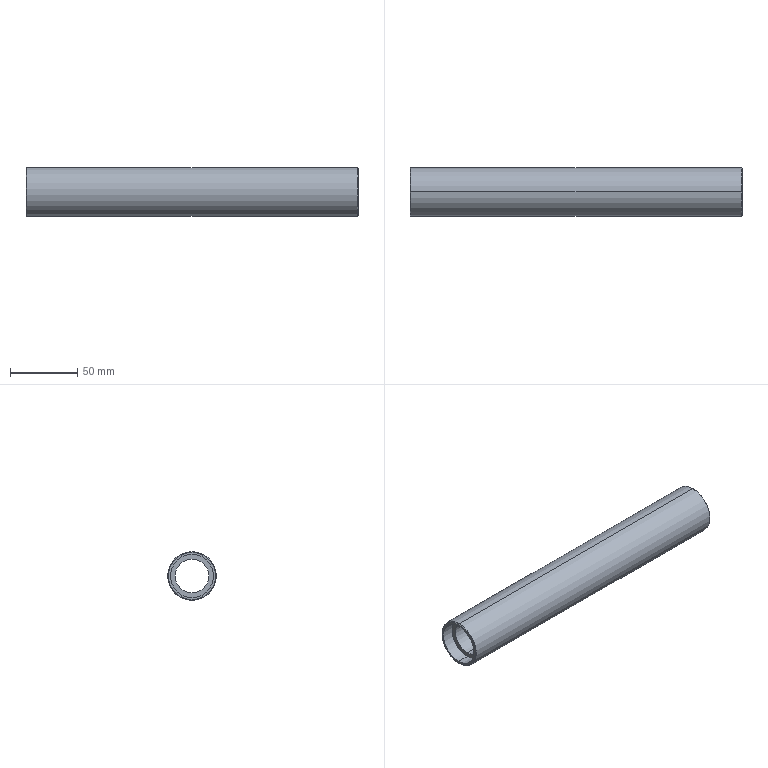Part | STEP file | 1 solid | 16 faces | box 246 x 36 x 36 mm | volume 123974 mm3 | cylinder 8 | cone 4 | plane 4 | commonest cylinder face diameters 32 x4 25 x2 36 x2
STEP:
#1=CARTESIAN_POINT('',(0.,0.,0.));
#2=DIRECTION('',(0.,0.,1.));
#3=DIRECTION('',(1.,0.,0.));
#4=AXIS2_PLACEMENT_3D('',#1,#2,#3);
#5=CARTESIAN_POINT('',(-123.,0.,17.5));
#6=VERTEX_POINT('',#5);
#7=CARTESIAN_POINT('',(-123.,0.,-17.5));
#8=VERTEX_POINT('',#7);
#9=CARTESIAN_POINT('',(-123.,0.,0.));
#10=DIRECTION('',(-1.,0.,0.));
#11=DIRECTION('',(0.,0.,-1.));
#12=AXIS2_PLACEMENT_3D('',#9,#10,#11);
#13=CIRCLE('',#12,17.5);
#14=CARTESIAN_POINT('',(-123.,0.,0.));
#15=DIRECTION('',(1.,0.,0.));
#16=DIRECTION('',(0.,0.,-1.));
#17=AXIS2_PLACEMENT_3D('',#14,#15,#16);
#18=CONICAL_SURFACE('',#17,17.5,0.7854);
#19=CARTESIAN_POINT('',(6.283,0.));
#20=DIRECTION('',(-1.,0.));
#21=VECTOR('',#20,1.);
#22=LINE('',#19,#21);
#23=(GEOMETRIC_REPRESENTATION_CONTEXT(2)PARAMETRIC_REPRESENTATION_CONTEXT()REPRESENTATION_CONTEXT('',''));
#24=DEFINITIONAL_REPRESENTATION('',(#22),#23);
#25=PCURVE('',#18,#24);
#26=CARTESIAN_POINT('',(-123.,18.,0.));
#27=DIRECTION('',(1.,0.,0.));
#28=DIRECTION('',(0.,0.,-1.));
#29=AXIS2_PLACEMENT_3D('',#26,#27,#28);
#30=PLANE('',#29);
#31=CARTESIAN_POINT('',(17.5,-18.));
#32=CARTESIAN_POINT('',(17.5,-48.311));
#33=CARTESIAN_POINT('',(-8.75,-33.155));
#34=CARTESIAN_POINT('',(-35.,-18.));
#35=CARTESIAN_POINT('',(-8.75,-2.845));
#36=CARTESIAN_POINT('',(17.5,12.311));
#37=CARTESIAN_POINT('',(17.5,-18.));
#38=(BOUNDED_CURVE()B_SPLINE_CURVE(2,(#31,#32,#33,#34,#35,#36,#37),.UNSPECIFIED.,.T.,.F.)B_SPLINE_CURVE_WITH_KNOTS((1,2,2,2,2,1),(-2.094,0.,2.094,4.189,6.283,8.378),.UNSPECIFIED.)CURVE()GEOMETRIC_REPRESENTATION_ITEM()RATIONAL_B_SPLINE_CURVE((1.,0.5,1.,0.5,1.,0.5,1.))REPRESENTATION_ITEM(''));
#39=(GEOMETRIC_REPRESENTATION_CONTEXT(2)PARAMETRIC_REPRESENTATION_CONTEXT()REPRESENTATION_CONTEXT('',''));
#40=DEFINITIONAL_REPRESENTATION('',(#38),#39);
#41=PCURVE('',#30,#40);
#42=SURFACE_CURVE('',#13,(#25,#41),.PCURVE_S1.);
#43=EDGE_CURVE('',#6,#8,#42,.T.);
#44=ORIENTED_EDGE('',*,*,#43,.F.);
#45=CARTESIAN_POINT('',(-122.5,0.,18.));
#46=VERTEX_POINT('',#45);
#47=CARTESIAN_POINT('',(-123.,0.,17.5));
#48=DIRECTION('',(0.7071,0.,0.7071));
#49=VECTOR('',#48,1.);
#50=LINE('',#47,#49);
#51=CARTESIAN_POINT('',(3.142,0.));
#52=DIRECTION('',(0.,1.));
#53=VECTOR('',#52,1.);
#54=LINE('',#51,#53);
#55=(GEOMETRIC_REPRESENTATION_CONTEXT(2)PARAMETRIC_REPRESENTATION_CONTEXT()REPRESENTATION_CONTEXT('',''));
#56=DEFINITIONAL_REPRESENTATION('',(#54),#55);
#57=PCURVE('',#18,#56);
#58=CARTESIAN_POINT('',(-123.,0.,0.));
#59=DIRECTION('',(1.,0.,0.));
#60=DIRECTION('',(0.,0.,-1.));
#61=AXIS2_PLACEMENT_3D('',#58,#59,#60);
#62=CONICAL_SURFACE('',#61,17.5,0.7854);
#63=CARTESIAN_POINT('',(3.142,0.));
#64=DIRECTION('',(0.,1.));
#65=VECTOR('',#64,1.);
#66=LINE('',#63,#65);
#67=(GEOMETRIC_REPRESENTATION_CONTEXT(2)PARAMETRIC_REPRESENTATION_CONTEXT()REPRESENTATION_CONTEXT('',''));
#68=DEFINITIONAL_REPRESENTATION('',(#66),#67);
#69=PCURVE('',#62,#68);
#70=SURFACE_CURVE('',#50,(#57,#69),.PCURVE_S1.);
#71=EDGE_CURVE('',#6,#46,#70,.T.);
#72=ORIENTED_EDGE('',*,*,#71,.T.);
#73=CARTESIAN_POINT('',(-122.5,0.,-18.));
#74=VERTEX_POINT('',#73);
#75=CARTESIAN_POINT('',(-122.5,0.,0.));
#76=DIRECTION('',(1.,0.,0.));
#77=DIRECTION('',(0.,0.,-1.));
#78=AXIS2_PLACEMENT_3D('',#75,#76,#77);
#79=CIRCLE('',#78,18.);
#80=CARTESIAN_POINT('',(0.,0.5));
#81=DIRECTION('',(1.,0.));
#82=VECTOR('',#81,1.);
#83=LINE('',#80,#82);
#84=(GEOMETRIC_REPRESENTATION_CONTEXT(2)PARAMETRIC_REPRESENTATION_CONTEXT()REPRESENTATION_CONTEXT('',''));
#85=DEFINITIONAL_REPRESENTATION('',(#83),#84);
#86=PCURVE('',#18,#85);
#87=CARTESIAN_POINT('',(0.,0.,0.));
#88=DIRECTION('',(-1.,0.,0.));
#89=DIRECTION('',(0.,0.,1.));
#90=AXIS2_PLACEMENT_3D('',#87,#88,#89);
#91=CYLINDRICAL_SURFACE('',#90,18.);
#92=CARTESIAN_POINT('',(3.142,122.5));
#93=DIRECTION('',(-1.,0.));
#94=VECTOR('',#93,1.);
#95=LINE('',#92,#94);
#96=(GEOMETRIC_REPRESENTATION_CONTEXT(2)PARAMETRIC_REPRESENTATION_CONTEXT()REPRESENTATION_CONTEXT('',''));
#97=DEFINITIONAL_REPRESENTATION('',(#95),#96);
#98=PCURVE('',#91,#97);
#99=SURFACE_CURVE('',#79,(#86,#98),.PCURVE_S1.);
#100=EDGE_CURVE('',#74,#46,#99,.T.);
#101=ORIENTED_EDGE('',*,*,#100,.F.);
#102=CARTESIAN_POINT('',(-123.,0.,-17.5));
#103=DIRECTION('',(0.7071,0.,-0.7071));
#104=VECTOR('',#103,1.);
#105=LINE('',#102,#104);
#106=CARTESIAN_POINT('',(0.,0.));
#107=DIRECTION('',(0.,1.));
#108=VECTOR('',#107,1.);
#109=LINE('',#106,#108);
#110=(GEOMETRIC_REPRESENTATION_CONTEXT(2)PARAMETRIC_REPRESENTATION_CONTEXT()REPRESENTATION_CONTEXT('',''));
#111=DEFINITIONAL_REPRESENTATION('',(#109),#110);
#112=PCURVE('',#18,#111);
#113=CARTESIAN_POINT('',(6.283,0.));
#114=DIRECTION('',(0.,1.));
#115=VECTOR('',#114,1.);
#116=LINE('',#113,#115);
#117=(GEOMETRIC_REPRESENTATION_CONTEXT(2)PARAMETRIC_REPRESENTATION_CONTEXT()REPRESENTATION_CONTEXT('',''));
#118=DEFINITIONAL_REPRESENTATION('',(#116),#117);
#119=PCURVE('',#62,#118);
#120=SURFACE_CURVE('',#105,(#112,#119),.PCURVE_S1.);
#121=EDGE_CURVE('',#8,#74,#120,.T.);
#122=ORIENTED_EDGE('',*,*,#121,.F.);
#123=EDGE_LOOP('',(#44,#72,#101,#122));
#124=FACE_BOUND('',#123,.T.);
#125=ADVANCED_FACE('',(#124),#18,.T.);
#126=CARTESIAN_POINT('',(123.,0.,-17.5));
#127=VERTEX_POINT('',#126);
#128=CARTESIAN_POINT('',(123.,0.,17.5));
#129=VERTEX_POINT('',#128);
#130=CARTESIAN_POINT('',(123.,0.,0.));
#131=DIRECTION('',(1.,0.,0.));
#132=DIRECTION('',(0.,0.,1.));
#133=AXIS2_PLACEMENT_3D('',#130,#131,#132);
#134=CIRCLE('',#133,17.5);
#135=CARTESIAN_POINT('',(122.5,0.,0.));
#136=DIRECTION('',(-1.,0.,0.));
#137=DIRECTION('',(0.,0.,1.));
#138=AXIS2_PLACEMENT_3D('',#135,#136,#137);
#139=CONICAL_SURFACE('',#138,18.,0.7854);
#140=CARTESIAN_POINT('',(6.283,-0.5));
#141=DIRECTION('',(-1.,0.));
#142=VECTOR('',#141,1.);
#143=LINE('',#140,#142);
#144=(GEOMETRIC_REPRESENTATION_CONTEXT(2)PARAMETRIC_REPRESENTATION_CONTEXT()REPRESENTATION_CONTEXT('',''));
#145=DEFINITIONAL_REPRESENTATION('',(#143),#144);
#146=PCURVE('',#139,#145);
#147=CARTESIAN_POINT('',(123.,18.,0.));
#148=DIRECTION('',(-1.,0.,0.));
#149=DIRECTION('',(0.,0.,1.));
#150=AXIS2_PLACEMENT_3D('',#147,#148,#149);
#151=PLANE('',#150);
#152=CARTESIAN_POINT('',(17.5,-18.));
#153=CARTESIAN_POINT('',(17.5,-48.311));
#154=CARTESIAN_POINT('',(-8.75,-33.155));
#155=CARTESIAN_POINT('',(-35.,-18.));
#156=CARTESIAN_POINT('',(-8.75,-2.845));
#157=CARTESIAN_POINT('',(17.5,12.311));
#158=CARTESIAN_POINT('',(17.5,-18.));
#159=(BOUNDED_CURVE()B_SPLINE_CURVE(2,(#152,#153,#154,#155,#156,#157,#158),.UNSPECIFIED.,.T.,.F.)B_SPLINE_CURVE_WITH_KNOTS((1,2,2,2,2,1),(-2.094,0.,2.094,4.189,6.283,8.378),.UNSPECIFIED.)CURVE()GEOMETRIC_REPRESENTATION_ITEM()RATIONAL_B_SPLINE_CURVE((1.,0.5,1.,0.5,1.,0.5,1.))REPRESENTATION_ITEM(''));
#160=(GEOMETRIC_REPRESENTATION_CONTEXT(2)PARAMETRIC_REPRESENTATION_CONTEXT()REPRESENTATION_CONTEXT('',''));
#161=DEFINITIONAL_REPRESENTATION('',(#159),#160);
#162=PCURVE('',#151,#161);
#163=SURFACE_CURVE('',#134,(#146,#162),.PCURVE_S1.);
#164=EDGE_CURVE('',#127,#129,#163,.T.);
#165=ORIENTED_EDGE('',*,*,#164,.F.);
#166=CARTESIAN_POINT('',(122.5,0.,-18.));
#167=VERTEX_POINT('',#166);
#168=CARTESIAN_POINT('',(122.5,0.,-18.));
#169=DIRECTION('',(-0.7071,0.,-0.7071));
#170=VECTOR('',#169,1.);
#171=LINE('',#168,#170);
#172=CARTESIAN_POINT('',(3.142,0.));
#173=DIRECTION('',(0.,1.));
#174=VECTOR('',#173,1.);
#175=LINE('',#172,#174);
#176=(GEOMETRIC_REPRESENTATION_CONTEXT(2)PARAMETRIC_REPRESENTATION_CONTEXT()REPRESENTATION_CONTEXT('',''));
#177=DEFINITIONAL_REPRESENTATION('',(#175),#176);
#178=PCURVE('',#139,#177);
#179=CARTESIAN_POINT('',(122.5,0.,0.));
#180=DIRECTION('',(-1.,0.,0.));
#181=DIRECTION('',(0.,0.,1.));
#182=AXIS2_PLACEMENT_3D('',#179,#180,#181);
#183=CONICAL_SURFACE('',#182,18.,0.7854);
#184=CARTESIAN_POINT('',(3.142,0.));
#185=DIRECTION('',(0.,1.));
#186=VECTOR('',#185,1.);
#187=LINE('',#184,#186);
#188=(GEOMETRIC_REPRESENTATION_CONTEXT(2)PARAMETRIC_REPRESENTATION_CONTEXT()REPRESENTATION_CONTEXT('',''));
#189=DEFINITIONAL_REPRESENTATION('',(#187),#188);
#190=PCURVE('',#183,#189);
#191=SURFACE_CURVE('',#171,(#178,#190),.PCURVE_S1.);
#192=EDGE_CURVE('',#127,#167,#191,.T.);
#193=ORIENTED_EDGE('',*,*,#192,.T.);
#194=CARTESIAN_POINT('',(122.5,0.,18.));
#195=VERTEX_POINT('',#194);
#196=CARTESIAN_POINT('',(122.5,0.,0.));
#197=DIRECTION('',(-1.,0.,0.));
#198=DIRECTION('',(0.,0.,1.));
#199=AXIS2_PLACEMENT_3D('',#196,#197,#198);
#200=CIRCLE('',#199,18.);
#201=CARTESIAN_POINT('',(0.,0.));
#202=DIRECTION('',(1.,0.));
#203=VECTOR('',#202,1.);
#204=LINE('',#201,#203);
#205=(GEOMETRIC_REPRESENTATION_CONTEXT(2)PARAMETRIC_REPRESENTATION_CONTEXT()REPRESENTATION_CONTEXT('',''));
#206=DEFINITIONAL_REPRESENTATION('',(#204),#205);
#207=PCURVE('',#139,#206);
#208=CARTESIAN_POINT('',(0.,-122.5));
#209=DIRECTION('',(1.,0.));
#210=VECTOR('',#209,1.);
#211=LINE('',#208,#210);
#212=(GEOMETRIC_REPRESENTATION_CONTEXT(2)PARAMETRIC_REPRESENTATION_CONTEXT()REPRESENTATION_CONTEXT('',''));
#213=DEFINITIONAL_REPRESENTATION('',(#211),#212);
#214=PCURVE('',#91,#213);
#215=SURFACE_CURVE('',#200,(#207,#214),.PCURVE_S1.);
#216=EDGE_CURVE('',#195,#167,#215,.T.);
#217=ORIENTED_EDGE('',*,*,#216,.F.);
#218=CARTESIAN_POINT('',(122.5,0.,18.));
#219=DIRECTION('',(-0.7071,0.,0.7071));
#220=VECTOR('',#219,1.);
#221=LINE('',#218,#220);
#222=CARTESIAN_POINT('',(0.,0.));
#223=DIRECTION('',(0.,1.));
#224=VECTOR('',#223,1.);
#225=LINE('',#222,#224);
#226=(GEOMETRIC_REPRESENTATION_CONTEXT(2)PARAMETRIC_REPRESENTATION_CONTEXT()REPRESENTATION_CONTEXT('',''));
#227=DEFINITIONAL_REPRESENTATION('',(#225),#226);
#228=PCURVE('',#139,#227);
#229=CARTESIAN_POINT('',(6.283,0.));
#230=DIRECTION('',(0.,1.));
#231=VECTOR('',#230,1.);
#232=LINE('',#229,#231);
#233=(GEOMETRIC_REPRESENTATION_CONTEXT(2)PARAMETRIC_REPRESENTATION_CONTEXT()REPRESENTATION_CONTEXT('',''));
#234=DEFINITIONAL_REPRESENTATION('',(#232),#233);
#235=PCURVE('',#183,#234);
#236=SURFACE_CURVE('',#221,(#228,#235),.PCURVE_S1.);
#237=EDGE_CURVE('',#129,#195,#236,.T.);
#238=ORIENTED_EDGE('',*,*,#237,.F.);
#239=EDGE_LOOP('',(#165,#193,#217,#238));
#240=FACE_BOUND('',#239,.T.);
#241=ADVANCED_FACE('',(#240),#139,.T.);
#242=CARTESIAN_POINT('',(114.,0.,12.5));
#243=VERTEX_POINT('',#242);
#244=CARTESIAN_POINT('',(-114.,0.,12.5));
#245=VERTEX_POINT('',#244);
#246=CARTESIAN_POINT('',(0.,0.,12.5));
#247=DIRECTION('',(-1.,0.,0.));
#248=VECTOR('',#247,1.);
#249=LINE('',#246,#248);
#250=CARTESIAN_POINT('',(0.,0.,0.));
#251=DIRECTION('',(-1.,0.,0.));
#252=DIRECTION('',(0.,0.,1.));
#253=AXIS2_PLACEMENT_3D('',#250,#251,#252);
#254=CYLINDRICAL_SURFACE('',#253,12.5);
#255=CARTESIAN_POINT('',(6.283,0.));
#256=DIRECTION('',(0.,1.));
#257=VECTOR('',#256,1.);
#258=LINE('',#255,#257);
#259=(GEOMETRIC_REPRESENTATION_CONTEXT(2)PARAMETRIC_REPRESENTATION_CONTEXT()REPRESENTATION_CONTEXT('',''));
#260=DEFINITIONAL_REPRESENTATION('',(#258),#259);
#261=PCURVE('',#254,#260);
#262=CARTESIAN_POINT('',(0.,0.,0.));
#263=DIRECTION('',(-1.,0.,0.));
#264=DIRECTION('',(0.,0.,1.));
#265=AXIS2_PLACEMENT_3D('',#262,#263,#264);
#266=CYLINDRICAL_SURFACE('',#265,12.5);
#267=CARTESIAN_POINT('',(0.,0.));
#268=DIRECTION('',(0.,1.));
#269=VECTOR('',#268,1.);
#270=LINE('',#267,#269);
#271=(GEOMETRIC_REPRESENTATION_CONTEXT(2)PARAMETRIC_REPRESENTATION_CONTEXT()REPRESENTATION_CONTEXT('',''));
#272=DEFINITIONAL_REPRESENTATION('',(#270),#271);
#273=PCURVE('',#266,#272);
#274=SURFACE_CURVE('',#249,(#261,#273),.PCURVE_S1.);
#275=EDGE_CURVE('',#243,#245,#274,.T.);
#276=ORIENTED_EDGE('',*,*,#275,.T.);
#277=CARTESIAN_POINT('',(-114.,0.,-12.5));
#278=VERTEX_POINT('',#277);
#279=CARTESIAN_POINT('',(-114.,0.,0.));
#280=DIRECTION('',(-1.,0.,0.));
#281=DIRECTION('',(0.,0.,1.));
#282=AXIS2_PLACEMENT_3D('',#279,#280,#281);
#283=CIRCLE('',#282,12.5);
#284=CARTESIAN_POINT('',(0.,114.));
#285=DIRECTION('',(1.,0.));
#286=VECTOR('',#285,1.);
#287=LINE('',#284,#286);
#288=(GEOMETRIC_REPRESENTATION_CONTEXT(2)PARAMETRIC_REPRESENTATION_CONTEXT()REPRESENTATION_CONTEXT('',''));
#289=DEFINITIONAL_REPRESENTATION('',(#287),#288);
#290=PCURVE('',#254,#289);
#291=CARTESIAN_POINT('',(-114.,16.,0.));
#292=DIRECTION('',(1.,0.,0.));
#293=DIRECTION('',(0.,0.,-1.));
#294=AXIS2_PLACEMENT_3D('',#291,#292,#293);
#295=PLANE('',#294);
#296=CARTESIAN_POINT('',(-12.5,-16.));
#297=CARTESIAN_POINT('',(-12.5,5.651));
#298=CARTESIAN_POINT('',(6.25,-5.175));
#299=CARTESIAN_POINT('',(25.,-16.));
#300=CARTESIAN_POINT('',(6.25,-26.825));
#301=CARTESIAN_POINT('',(-12.5,-37.651));
#302=CARTESIAN_POINT('',(-12.5,-16.));
#303=(BOUNDED_CURVE()B_SPLINE_CURVE(2,(#296,#297,#298,#299,#300,#301,#302),.UNSPECIFIED.,.T.,.F.)B_SPLINE_CURVE_WITH_KNOTS((1,2,2,2,2,1),(-2.094,0.,2.094,4.189,6.283,8.378),.UNSPECIFIED.)CURVE()GEOMETRIC_REPRESENTATION_ITEM()RATIONAL_B_SPLINE_CURVE((1.,0.5,1.,0.5,1.,0.5,1.))REPRESENTATION_ITEM(''));
#304=(GEOMETRIC_REPRESENTATION_CONTEXT(2)PARAMETRIC_REPRESENTATION_CONTEXT()REPRESENTATION_CONTEXT('',''));
#305=DEFINITIONAL_REPRESENTATION('',(#303),#304);
#306=PCURVE('',#295,#305);
#307=SURFACE_CURVE('',#283,(#290,#306),.PCURVE_S1.);
#308=EDGE_CURVE('',#278,#245,#307,.T.);
#309=ORIENTED_EDGE('',*,*,#308,.F.);
#310=CARTESIAN_POINT('',(114.,0.,-12.5));
#311=VERTEX_POINT('',#310);
#312=CARTESIAN_POINT('',(0.,0.,-12.5));
#313=DIRECTION('',(-1.,0.,0.));
#314=VECTOR('',#313,1.);
#315=LINE('',#312,#314);
#316=CARTESIAN_POINT('',(3.142,0.));
#317=DIRECTION('',(0.,1.));
#318=VECTOR('',#317,1.);
#319=LINE('',#316,#318);
#320=(GEOMETRIC_REPRESENTATION_CONTEXT(2)PARAMETRIC_REPRESENTATION_CONTEXT()REPRESENTATION_CONTEXT('',''));
#321=DEFINITIONAL_REPRESENTATION('',(#319),#320);
#322=PCURVE('',#254,#321);
#323=CARTESIAN_POINT('',(3.142,0.));
#324=DIRECTION('',(0.,1.));
#325=VECTOR('',#324,1.);
#326=LINE('',#323,#325);
#327=(GEOMETRIC_REPRESENTATION_CONTEXT(2)PARAMETRIC_REPRESENTATION_CONTEXT()REPRESENTATION_CONTEXT('',''));
#328=DEFINITIONAL_REPRESENTATION('',(#326),#327);
#329=PCURVE('',#266,#328);
#330=SURFACE_CURVE('',#315,(#322,#329),.PCURVE_S1.);
#331=EDGE_CURVE('',#311,#278,#330,.T.);
#332=ORIENTED_EDGE('',*,*,#331,.F.);
#333=CARTESIAN_POINT('',(114.,0.,0.));
#334=DIRECTION('',(-1.,0.,0.));
#335=DIRECTION('',(0.,0.,1.));
#336=AXIS2_PLACEMENT_3D('',#333,#334,#335);
#337=CIRCLE('',#336,12.5);
#338=CARTESIAN_POINT('',(0.,-114.));
#339=DIRECTION('',(1.,0.));
#340=VECTOR('',#339,1.);
#341=LINE('',#338,#340);
#342=(GEOMETRIC_REPRESENTATION_CONTEXT(2)PARAMETRIC_REPRESENTATION_CONTEXT()REPRESENTATION_CONTEXT('',''));
#343=DEFINITIONAL_REPRESENTATION('',(#341),#342);
#344=PCURVE('',#254,#343);
#345=CARTESIAN_POINT('',(114.,16.,0.));
#346=DIRECTION('',(-1.,0.,0.));
#347=DIRECTION('',(0.,0.,1.));
#348=AXIS2_PLACEMENT_3D('',#345,#346,#347);
#349=PLANE('',#348);
#350=CARTESIAN_POINT('',(0.,-16.));
#351=DIRECTION('',(1.,0.));
#352=AXIS2_PLACEMENT_2D('',#350,#351);
#353=CIRCLE('',#352,12.5);
#354=(GEOMETRIC_REPRESENTATION_CONTEXT(2)PARAMETRIC_REPRESENTATION_CONTEXT()REPRESENTATION_CONTEXT('',''));
#355=DEFINITIONAL_REPRESENTATION('',(#353),#354);
#356=PCURVE('',#349,#355);
#357=SURFACE_CURVE('',#337,(#344,#356),.PCURVE_S1.);
#358=EDGE_CURVE('',#311,#243,#357,.T.);
#359=ORIENTED_EDGE('',*,*,#358,.T.);
#360=EDGE_LOOP('',(#276,#309,#332,#359));
#361=FACE_BOUND('',#360,.F.);
#362=ADVANCED_FACE('',(#361),#254,.F.);
#363=CARTESIAN_POINT('',(123.,0.,16.));
#364=VERTEX_POINT('',#363);
#365=CARTESIAN_POINT('',(114.,0.,16.));
#366=VERTEX_POINT('',#365);
#367=CARTESIAN_POINT('',(0.,0.,16.));
#368=DIRECTION('',(-1.,0.,0.));
#369=VECTOR('',#368,1.);
#370=LINE('',#367,#369);
#371=CARTESIAN_POINT('',(0.,0.,0.));
#372=DIRECTION('',(-1.,0.,0.));
#373=DIRECTION('',(0.,0.,1.));
#374=AXIS2_PLACEMENT_3D('',#371,#372,#373);
#375=CYLINDRICAL_SURFACE('',#374,16.);
#376=CARTESIAN_POINT('',(6.283,0.));
#377=DIRECTION('',(0.,1.));
#378=VECTOR('',#377,1.);
#379=LINE('',#376,#378);
#380=(GEOMETRIC_REPRESENTATION_CONTEXT(2)PARAMETRIC_REPRESENTATION_CONTEXT()REPRESENTATION_CONTEXT('',''));
#381=DEFINITIONAL_REPRESENTATION('',(#379),#380);
#382=PCURVE('',#375,#381);
#383=CARTESIAN_POINT('',(0.,0.,0.));
#384=DIRECTION('',(-1.,0.,0.));
#385=DIRECTION('',(0.,0.,1.));
#386=AXIS2_PLACEMENT_3D('',#383,#384,#385);
#387=CYLINDRICAL_SURFACE('',#386,16.);
#388=CARTESIAN_POINT('',(0.,0.));
#389=DIRECTION('',(0.,1.));
#390=VECTOR('',#389,1.);
#391=LINE('',#388,#390);
#392=(GEOMETRIC_REPRESENTATION_CONTEXT(2)PARAMETRIC_REPRESENTATION_CONTEXT()REPRESENTATION_CONTEXT('',''));
#393=DEFINITIONAL_REPRESENTATION('',(#391),#392);
#394=PCURVE('',#387,#393);
#395=SURFACE_CURVE('',#370,(#382,#394),.PCURVE_S1.);
#396=EDGE_CURVE('',#364,#366,#395,.T.);
#397=ORIENTED_EDGE('',*,*,#396,.T.);
#398=CARTESIAN_POINT('',(114.,0.,-16.));
#399=VERTEX_POINT('',#398);
#400=CARTESIAN_POINT('',(114.,0.,0.));
#401=DIRECTION('',(-1.,0.,0.));
#402=DIRECTION('',(0.,0.,1.));
#403=AXIS2_PLACEMENT_3D('',#400,#401,#402);
#404=CIRCLE('',#403,16.);
#405=CARTESIAN_POINT('',(0.,-114.));
#406=DIRECTION('',(1.,0.));
#407=VECTOR('',#406,1.);
#408=LINE('',#405,#407);
#409=(GEOMETRIC_REPRESENTATION_CONTEXT(2)PARAMETRIC_REPRESENTATION_CONTEXT()REPRESENTATION_CONTEXT('',''));
#410=DEFINITIONAL_REPRESENTATION('',(#408),#409);
#411=PCURVE('',#375,#410);
#412=CARTESIAN_POINT('',(0.,-16.));
#413=DIRECTION('',(1.,0.));
#414=AXIS2_PLACEMENT_2D('',#412,#413);
#415=CIRCLE('',#414,16.);
#416=(GEOMETRIC_REPRESENTATION_CONTEXT(2)PARAMETRIC_REPRESENTATION_CONTEXT()REPRESENTATION_CONTEXT('',''));
#417=DEFINITIONAL_REPRESENTATION('',(#415),#416);
#418=PCURVE('',#349,#417);
#419=SURFACE_CURVE('',#404,(#411,#418),.PCURVE_S1.);
#420=EDGE_CURVE('',#399,#366,#419,.T.);
#421=ORIENTED_EDGE('',*,*,#420,.F.);
#422=CARTESIAN_POINT('',(123.,0.,-16.));
#423=VERTEX_POINT('',#422);
#424=CARTESIAN_POINT('',(0.,0.,-16.));
#425=DIRECTION('',(-1.,0.,0.));
#426=VECTOR('',#425,1.);
#427=LINE('',#424,#426);
#428=CARTESIAN_POINT('',(3.142,0.));
#429=DIRECTION('',(0.,1.));
#430=VECTOR('',#429,1.);
#431=LINE('',#428,#430);
#432=(GEOMETRIC_REPRESENTATION_CONTEXT(2)PARAMETRIC_REPRESENTATION_CONTEXT()REPRESENTATION_CONTEXT('',''));
#433=DEFINITIONAL_REPRESENTATION('',(#431),#432);
#434=PCURVE('',#375,#433);
#435=CARTESIAN_POINT('',(3.142,0.));
#436=DIRECTION('',(0.,1.));
#437=VECTOR('',#436,1.);
#438=LINE('',#435,#437);
#439=(GEOMETRIC_REPRESENTATION_CONTEXT(2)PARAMETRIC_REPRESENTATION_CONTEXT()REPRESENTATION_CONTEXT('',''));
#440=DEFINITIONAL_REPRESENTATION('',(#438),#439);
#441=PCURVE('',#387,#440);
#442=SURFACE_CURVE('',#427,(#434,#441),.PCURVE_S1.);
#443=EDGE_CURVE('',#423,#399,#442,.T.);
#444=ORIENTED_EDGE('',*,*,#443,.F.);
#445=CARTESIAN_POINT('',(123.,0.,0.));
#446=DIRECTION('',(-1.,0.,0.));
#447=DIRECTION('',(0.,0.,1.));
#448=AXIS2_PLACEMENT_3D('',#445,#446,#447);
#449=CIRCLE('',#448,16.);
#450=CARTESIAN_POINT('',(0.,-123.));
#451=DIRECTION('',(1.,0.));
#452=VECTOR('',#451,1.);
#453=LINE('',#450,#452);
#454=(GEOMETRIC_REPRESENTATION_CONTEXT(2)PARAMETRIC_REPRESENTATION_CONTEXT()REPRESENTATION_CONTEXT('',''));
#455=DEFINITIONAL_REPRESENTATION('',(#453),#454);
#456=PCURVE('',#375,#455);
#457=CARTESIAN_POINT('',(0.,-18.));
#458=DIRECTION('',(1.,0.));
#459=AXIS2_PLACEMENT_2D('',#457,#458);
#460=CIRCLE('',#459,16.);
#461=(GEOMETRIC_REPRESENTATION_CONTEXT(2)PARAMETRIC_REPRESENTATION_CONTEXT()REPRESENTATION_CONTEXT('',''));
#462=DEFINITIONAL_REPRESENTATION('',(#460),#461);
#463=PCURVE('',#151,#462);
#464=SURFACE_CURVE('',#449,(#456,#463),.PCURVE_S1.);
#465=EDGE_CURVE('',#423,#364,#464,.T.);
#466=ORIENTED_EDGE('',*,*,#465,.T.);
#467=EDGE_LOOP('',(#397,#421,#444,#466));
#468=FACE_BOUND('',#467,.F.);
#469=ADVANCED_FACE('',(#468),#375,.F.);
#470=ORIENTED_EDGE('',*,*,#216,.T.);
#471=CARTESIAN_POINT('',(0.,0.,-18.));
#472=DIRECTION('',(-1.,0.,0.));
#473=VECTOR('',#472,1.);
#474=LINE('',#471,#473);
#475=CARTESIAN_POINT('',(3.142,0.));
#476=DIRECTION('',(0.,1.));
#477=VECTOR('',#476,1.);
#478=LINE('',#475,#477);
#479=(GEOMETRIC_REPRESENTATION_CONTEXT(2)PARAMETRIC_REPRESENTATION_CONTEXT()REPRESENTATION_CONTEXT('',''));
#480=DEFINITIONAL_REPRESENTATION('',(#478),#479);
#481=PCURVE('',#91,#480);
#482=CARTESIAN_POINT('',(0.,0.,0.));
#483=DIRECTION('',(-1.,0.,0.));
#484=DIRECTION('',(0.,0.,1.));
#485=AXIS2_PLACEMENT_3D('',#482,#483,#484);
#486=CYLINDRICAL_SURFACE('',#485,18.);
#487=CARTESIAN_POINT('',(3.142,0.));
#488=DIRECTION('',(0.,1.));
#489=VECTOR('',#488,1.);
#490=LINE('',#487,#489);
#491=(GEOMETRIC_REPRESENTATION_CONTEXT(2)PARAMETRIC_REPRESENTATION_CONTEXT()REPRESENTATION_CONTEXT('',''));
#492=DEFINITIONAL_REPRESENTATION('',(#490),#491);
#493=PCURVE('',#486,#492);
#494=SURFACE_CURVE('',#474,(#481,#493),.PCURVE_S1.);
#495=EDGE_CURVE('',#167,#74,#494,.T.);
#496=ORIENTED_EDGE('',*,*,#495,.T.);
#497=ORIENTED_EDGE('',*,*,#100,.T.);
#498=CARTESIAN_POINT('',(0.,0.,18.));
#499=DIRECTION('',(-1.,0.,0.));
#500=VECTOR('',#499,1.);
#501=LINE('',#498,#500);
#502=CARTESIAN_POINT('',(0.,0.));
#503=DIRECTION('',(0.,1.));
#504=VECTOR('',#503,1.);
#505=LINE('',#502,#504);
#506=(GEOMETRIC_REPRESENTATION_CONTEXT(2)PARAMETRIC_REPRESENTATION_CONTEXT()REPRESENTATION_CONTEXT('',''));
#507=DEFINITIONAL_REPRESENTATION('',(#505),#506);
#508=PCURVE('',#91,#507);
#509=CARTESIAN_POINT('',(6.283,0.));
#510=DIRECTION('',(0.,1.));
#511=VECTOR('',#510,1.);
#512=LINE('',#509,#511);
#513=(GEOMETRIC_REPRESENTATION_CONTEXT(2)PARAMETRIC_REPRESENTATION_CONTEXT()REPRESENTATION_CONTEXT('',''));
#514=DEFINITIONAL_REPRESENTATION('',(#512),#513);
#515=PCURVE('',#486,#514);
#516=SURFACE_CURVE('',#501,(#508,#515),.PCURVE_S1.);
#517=EDGE_CURVE('',#195,#46,#516,.T.);
#518=ORIENTED_EDGE('',*,*,#517,.F.);
#519=EDGE_LOOP('',(#470,#496,#497,#518));
#520=FACE_BOUND('',#519,.T.);
#521=ADVANCED_FACE('',(#520),#91,.T.);
#522=CARTESIAN_POINT('',(-114.,0.,16.));
#523=VERTEX_POINT('',#522);
#524=CARTESIAN_POINT('',(-123.,0.,16.));
#525=VERTEX_POINT('',#524);
#526=CARTESIAN_POINT('',(0.,0.,16.));
#527=DIRECTION('',(-1.,0.,0.));
#528=VECTOR('',#527,1.);
#529=LINE('',#526,#528);
#530=CARTESIAN_POINT('',(0.,0.,0.));
#531=DIRECTION('',(-1.,0.,0.));
#532=DIRECTION('',(0.,0.,1.));
#533=AXIS2_PLACEMENT_3D('',#530,#531,#532);
#534=CYLINDRICAL_SURFACE('',#533,16.);
#535=CARTESIAN_POINT('',(6.283,0.));
#536=DIRECTION('',(0.,1.));
#537=VECTOR('',#536,1.);
#538=LINE('',#535,#537);
#539=(GEOMETRIC_REPRESENTATION_CONTEXT(2)PARAMETRIC_REPRESENTATION_CONTEXT()REPRESENTATION_CONTEXT('',''));
#540=DEFINITIONAL_REPRESENTATION('',(#538),#539);
#541=PCURVE('',#534,#540);
#542=CARTESIAN_POINT('',(0.,0.,0.));
#543=DIRECTION('',(-1.,0.,0.));
#544=DIRECTION('',(0.,0.,1.));
#545=AXIS2_PLACEMENT_3D('',#542,#543,#544);
#546=CYLINDRICAL_SURFACE('',#545,16.);
#547=CARTESIAN_POINT('',(0.,0.));
#548=DIRECTION('',(0.,1.));
#549=VECTOR('',#548,1.);
#550=LINE('',#547,#549);
#551=(GEOMETRIC_REPRESENTATION_CONTEXT(2)PARAMETRIC_REPRESENTATION_CONTEXT()REPRESENTATION_CONTEXT('',''));
#552=DEFINITIONAL_REPRESENTATION('',(#550),#551);
#553=PCURVE('',#546,#552);
#554=SURFACE_CURVE('',#529,(#541,#553),.PCURVE_S1.);
#555=EDGE_CURVE('',#523,#525,#554,.T.);
#556=ORIENTED_EDGE('',*,*,#555,.T.);
#557=CARTESIAN_POINT('',(-123.,0.,-16.));
#558=VERTEX_POINT('',#557);
#559=CARTESIAN_POINT('',(-123.,0.,0.));
#560=DIRECTION('',(-1.,0.,0.));
#561=DIRECTION('',(0.,0.,1.));
#562=AXIS2_PLACEMENT_3D('',#559,#560,#561);
#563=CIRCLE('',#562,16.);
#564=CARTESIAN_POINT('',(0.,123.));
#565=DIRECTION('',(1.,0.));
#566=VECTOR('',#565,1.);
#567=LINE('',#564,#566);
#568=(GEOMETRIC_REPRESENTATION_CONTEXT(2)PARAMETRIC_REPRESENTATION_CONTEXT()REPRESENTATION_CONTEXT('',''));
#569=DEFINITIONAL_REPRESENTATION('',(#567),#568);
#570=PCURVE('',#534,#569);
#571=CARTESIAN_POINT('',(-16.,-18.));
#572=CARTESIAN_POINT('',(-16.,9.713));
#573=CARTESIAN_POINT('',(8.,-4.144));
#574=CARTESIAN_POINT('',(32.,-18.));
#575=CARTESIAN_POINT('',(8.,-31.856));
#576=CARTESIAN_POINT('',(-16.,-45.713));
#577=CARTESIAN_POINT('',(-16.,-18.));
#578=(BOUNDED_CURVE()B_SPLINE_CURVE(2,(#571,#572,#573,#574,#575,#576,#577),.UNSPECIFIED.,.T.,.F.)B_SPLINE_CURVE_WITH_KNOTS((1,2,2,2,2,1),(-2.094,0.,2.094,4.189,6.283,8.378),.UNSPECIFIED.)CURVE()GEOMETRIC_REPRESENTATION_ITEM()RATIONAL_B_SPLINE_CURVE((1.,0.5,1.,0.5,1.,0.5,1.))REPRESENTATION_ITEM(''));
#579=(GEOMETRIC_REPRESENTATION_CONTEXT(2)PARAMETRIC_REPRESENTATION_CONTEXT()REPRESENTATION_CONTEXT('',''));
#580=DEFINITIONAL_REPRESENTATION('',(#578),#579);
#581=PCURVE('',#30,#580);
#582=SURFACE_CURVE('',#563,(#570,#581),.PCURVE_S1.);
#583=EDGE_CURVE('',#558,#525,#582,.T.);
#584=ORIENTED_EDGE('',*,*,#583,.F.);
#585=CARTESIAN_POINT('',(-114.,0.,-16.));
#586=VERTEX_POINT('',#585);
#587=CARTESIAN_POINT('',(0.,0.,-16.));
#588=DIRECTION('',(-1.,0.,0.));
#589=VECTOR('',#588,1.);
#590=LINE('',#587,#589);
#591=CARTESIAN_POINT('',(3.142,0.));
#592=DIRECTION('',(0.,1.));
#593=VECTOR('',#592,1.);
#594=LINE('',#591,#593);
#595=(GEOMETRIC_REPRESENTATION_CONTEXT(2)PARAMETRIC_REPRESENTATION_CONTEXT()REPRESENTATION_CONTEXT('',''));
#596=DEFINITIONAL_REPRESENTATION('',(#594),#595);
#597=PCURVE('',#534,#596);
#598=CARTESIAN_POINT('',(3.142,0.));
#599=DIRECTION('',(0.,1.));
#600=VECTOR('',#599,1.);
#601=LINE('',#598,#600);
#602=(GEOMETRIC_REPRESENTATION_CONTEXT(2)PARAMETRIC_REPRESENTATION_CONTEXT()REPRESENTATION_CONTEXT('',''));
#603=DEFINITIONAL_REPRESENTATION('',(#601),#602);
#604=PCURVE('',#546,#603);
#605=SURFACE_CURVE('',#590,(#597,#604),.PCURVE_S1.);
#606=EDGE_CURVE('',#586,#558,#605,.T.);
#607=ORIENTED_EDGE('',*,*,#606,.F.);
#608=CARTESIAN_POINT('',(-114.,0.,0.));
#609=DIRECTION('',(-1.,0.,0.));
#610=DIRECTION('',(0.,0.,1.));
#611=AXIS2_PLACEMENT_3D('',#608,#609,#610);
#612=CIRCLE('',#611,16.);
#613=CARTESIAN_POINT('',(0.,114.));
#614=DIRECTION('',(1.,0.));
#615=VECTOR('',#614,1.);
#616=LINE('',#613,#615);
#617=(GEOMETRIC_REPRESENTATION_CONTEXT(2)PARAMETRIC_REPRESENTATION_CONTEXT()REPRESENTATION_CONTEXT('',''));
#618=DEFINITIONAL_REPRESENTATION('',(#616),#617);
#619=PCURVE('',#534,#618);
#620=CARTESIAN_POINT('',(-16.,-16.));
#621=CARTESIAN_POINT('',(-16.,11.713));
#622=CARTESIAN_POINT('',(8.,-2.144));
#623=CARTESIAN_POINT('',(32.,-16.));
#624=CARTESIAN_POINT('',(8.,-29.856));
#625=CARTESIAN_POINT('',(-16.,-43.713));
#626=CARTESIAN_POINT('',(-16.,-16.));
#627=(BOUNDED_CURVE()B_SPLINE_CURVE(2,(#620,#621,#622,#623,#624,#625,#626),.UNSPECIFIED.,.T.,.F.)B_SPLINE_CURVE_WITH_KNOTS((1,2,2,2,2,1),(-2.094,0.,2.094,4.189,6.283,8.378),.UNSPECIFIED.)CURVE()GEOMETRIC_REPRESENTATION_ITEM()RATIONAL_B_SPLINE_CURVE((1.,0.5,1.,0.5,1.,0.5,1.))REPRESENTATION_ITEM(''));
#628=(GEOMETRIC_REPRESENTATION_CONTEXT(2)PARAMETRIC_REPRESENTATION_CONTEXT()REPRESENTATION_CONTEXT('',''));
#629=DEFINITIONAL_REPRESENTATION('',(#627),#628);
#630=PCURVE('',#295,#629);
#631=SURFACE_CURVE('',#612,(#619,#630),.PCURVE_S1.);
#632=EDGE_CURVE('',#586,#523,#631,.T.);
#633=ORIENTED_EDGE('',*,*,#632,.T.);
#634=EDGE_LOOP('',(#556,#584,#607,#633));
#635=FACE_BOUND('',#634,.F.);
#636=ADVANCED_FACE('',(#635),#534,.F.);
#637=CARTESIAN_POINT('',(-114.,0.,0.));
#638=DIRECTION('',(-1.,0.,0.));
#639=DIRECTION('',(0.,0.,1.));
#640=AXIS2_PLACEMENT_3D('',#637,#638,#639);
#641=CIRCLE('',#640,12.5);
#642=CARTESIAN_POINT('',(-12.5,-16.));
#643=CARTESIAN_POINT('',(-12.5,5.651));
#644=CARTESIAN_POINT('',(6.25,-5.175));
#645=CARTESIAN_POINT('',(25.,-16.));
#646=CARTESIAN_POINT('',(6.25,-26.825));
#647=CARTESIAN_POINT('',(-12.5,-37.651));
#648=CARTESIAN_POINT('',(-12.5,-16.));
#649=(BOUNDED_CURVE()B_SPLINE_CURVE(2,(#642,#643,#644,#645,#646,#647,#648),.UNSPECIFIED.,.T.,.F.)B_SPLINE_CURVE_WITH_KNOTS((1,2,2,2,2,1),(-2.094,0.,2.094,4.189,6.283,8.378),.UNSPECIFIED.)CURVE()GEOMETRIC_REPRESENTATION_ITEM()RATIONAL_B_SPLINE_CURVE((1.,0.5,1.,0.5,1.,0.5,1.))REPRESENTATION_ITEM(''));
#650=(GEOMETRIC_REPRESENTATION_CONTEXT(2)PARAMETRIC_REPRESENTATION_CONTEXT()REPRESENTATION_CONTEXT('',''));
#651=DEFINITIONAL_REPRESENTATION('',(#649),#650);
#652=PCURVE('',#295,#651);
#653=CARTESIAN_POINT('',(0.,114.));
#654=DIRECTION('',(1.,0.));
#655=VECTOR('',#654,1.);
#656=LINE('',#653,#655);
#657=(GEOMETRIC_REPRESENTATION_CONTEXT(2)PARAMETRIC_REPRESENTATION_CONTEXT()REPRESENTATION_CONTEXT('',''));
#658=DEFINITIONAL_REPRESENTATION('',(#656),#657);
#659=PCURVE('',#266,#658);
#660=SURFACE_CURVE('',#641,(#652,#659),.PCURVE_S1.);
#661=EDGE_CURVE('',#245,#278,#660,.T.);
#662=ORIENTED_EDGE('',*,*,#661,.F.);
#663=ORIENTED_EDGE('',*,*,#308,.F.);
#664=EDGE_LOOP('',(#662,#663));
#665=FACE_BOUND('',#664,.T.);
#666=CARTESIAN_POINT('',(-114.,0.,0.));
#667=DIRECTION('',(-1.,0.,0.));
#668=DIRECTION('',(0.,0.,1.));
#669=AXIS2_PLACEMENT_3D('',#666,#667,#668);
#670=CIRCLE('',#669,16.);
#671=CARTESIAN_POINT('',(-16.,-16.));
#672=CARTESIAN_POINT('',(-16.,11.713));
#673=CARTESIAN_POINT('',(8.,-2.144));
#674=CARTESIAN_POINT('',(32.,-16.));
#675=CARTESIAN_POINT('',(8.,-29.856));
#676=CARTESIAN_POINT('',(-16.,-43.713));
#677=CARTESIAN_POINT('',(-16.,-16.));
#678=(BOUNDED_CURVE()B_SPLINE_CURVE(2,(#671,#672,#673,#674,#675,#676,#677),.UNSPECIFIED.,.T.,.F.)B_SPLINE_CURVE_WITH_KNOTS((1,2,2,2,2,1),(-2.094,0.,2.094,4.189,6.283,8.378),.UNSPECIFIED.)CURVE()GEOMETRIC_REPRESENTATION_ITEM()RATIONAL_B_SPLINE_CURVE((1.,0.5,1.,0.5,1.,0.5,1.))REPRESENTATION_ITEM(''));
#679=(GEOMETRIC_REPRESENTATION_CONTEXT(2)PARAMETRIC_REPRESENTATION_CONTEXT()REPRESENTATION_CONTEXT('',''));
#680=DEFINITIONAL_REPRESENTATION('',(#678),#679);
#681=PCURVE('',#295,#680);
#682=CARTESIAN_POINT('',(0.,114.));
#683=DIRECTION('',(1.,0.));
#684=VECTOR('',#683,1.);
#685=LINE('',#682,#684);
#686=(GEOMETRIC_REPRESENTATION_CONTEXT(2)PARAMETRIC_REPRESENTATION_CONTEXT()REPRESENTATION_CONTEXT('',''));
#687=DEFINITIONAL_REPRESENTATION('',(#685),#686);
#688=PCURVE('',#546,#687);
#689=SURFACE_CURVE('',#670,(#681,#688),.PCURVE_S1.);
#690=EDGE_CURVE('',#523,#586,#689,.T.);
#691=ORIENTED_EDGE('',*,*,#690,.T.);
#692=ORIENTED_EDGE('',*,*,#632,.T.);
#693=EDGE_LOOP('',(#691,#692));
#694=FACE_BOUND('',#693,.T.);
#695=ADVANCED_FACE('',(#665,#694),#295,.F.);
#696=CARTESIAN_POINT('',(-123.,0.,0.));
#697=DIRECTION('',(-1.,0.,0.));
#698=DIRECTION('',(0.,0.,1.));
#699=AXIS2_PLACEMENT_3D('',#696,#697,#698);
#700=CIRCLE('',#699,16.);
#701=CARTESIAN_POINT('',(0.,123.));
#702=DIRECTION('',(1.,0.));
#703=VECTOR('',#702,1.);
#704=LINE('',#701,#703);
#705=(GEOMETRIC_REPRESENTATION_CONTEXT(2)PARAMETRIC_REPRESENTATION_CONTEXT()REPRESENTATION_CONTEXT('',''));
#706=DEFINITIONAL_REPRESENTATION('',(#704),#705);
#707=PCURVE('',#546,#706);
#708=CARTESIAN_POINT('',(-16.,-18.));
#709=CARTESIAN_POINT('',(-16.,9.713));
#710=CARTESIAN_POINT('',(8.,-4.144));
#711=CARTESIAN_POINT('',(32.,-18.));
#712=CARTESIAN_POINT('',(8.,-31.856));
#713=CARTESIAN_POINT('',(-16.,-45.713));
#714=CARTESIAN_POINT('',(-16.,-18.));
#715=(BOUNDED_CURVE()B_SPLINE_CURVE(2,(#708,#709,#710,#711,#712,#713,#714),.UNSPECIFIED.,.T.,.F.)B_SPLINE_CURVE_WITH_KNOTS((1,2,2,2,2,1),(-2.094,0.,2.094,4.189,6.283,8.378),.UNSPECIFIED.)CURVE()GEOMETRIC_REPRESENTATION_ITEM()RATIONAL_B_SPLINE_CURVE((1.,0.5,1.,0.5,1.,0.5,1.))REPRESENTATION_ITEM(''));
#716=(GEOMETRIC_REPRESENTATION_CONTEXT(2)PARAMETRIC_REPRESENTATION_CONTEXT()REPRESENTATION_CONTEXT('',''));
#717=DEFINITIONAL_REPRESENTATION('',(#715),#716);
#718=PCURVE('',#30,#717);
#719=SURFACE_CURVE('',#700,(#707,#718),.PCURVE_S1.);
#720=EDGE_CURVE('',#525,#558,#719,.T.);
#721=ORIENTED_EDGE('',*,*,#720,.F.);
#722=ORIENTED_EDGE('',*,*,#555,.F.);
#723=ORIENTED_EDGE('',*,*,#690,.T.);
#724=ORIENTED_EDGE('',*,*,#606,.T.);
#725=EDGE_LOOP('',(#721,#722,#723,#724));
#726=FACE_BOUND('',#725,.F.);
#727=ADVANCED_FACE('',(#726),#546,.F.);
#728=CARTESIAN_POINT('',(-123.,0.,0.));
#729=DIRECTION('',(-1.,0.,0.));
#730=DIRECTION('',(0.,0.,-1.));
#731=AXIS2_PLACEMENT_3D('',#728,#729,#730);
#732=CIRCLE('',#731,17.5);
#733=CARTESIAN_POINT('',(17.5,-18.));
#734=CARTESIAN_POINT('',(17.5,-48.311));
#735=CARTESIAN_POINT('',(-8.75,-33.155));
#736=CARTESIAN_POINT('',(-35.,-18.));
#737=CARTESIAN_POINT('',(-8.75,-2.845));
#738=CARTESIAN_POINT('',(17.5,12.311));
#739=CARTESIAN_POINT('',(17.5,-18.));
#740=(BOUNDED_CURVE()B_SPLINE_CURVE(2,(#733,#734,#735,#736,#737,#738,#739),.UNSPECIFIED.,.T.,.F.)B_SPLINE_CURVE_WITH_KNOTS((1,2,2,2,2,1),(-2.094,0.,2.094,4.189,6.283,8.378),.UNSPECIFIED.)CURVE()GEOMETRIC_REPRESENTATION_ITEM()RATIONAL_B_SPLINE_CURVE((1.,0.5,1.,0.5,1.,0.5,1.))REPRESENTATION_ITEM(''));
#741=(GEOMETRIC_REPRESENTATION_CONTEXT(2)PARAMETRIC_REPRESENTATION_CONTEXT()REPRESENTATION_CONTEXT('',''));
#742=DEFINITIONAL_REPRESENTATION('',(#740),#741);
#743=PCURVE('',#30,#742);
#744=CARTESIAN_POINT('',(6.283,0.));
#745=DIRECTION('',(-1.,0.));
#746=VECTOR('',#745,1.);
#747=LINE('',#744,#746);
#748=(GEOMETRIC_REPRESENTATION_CONTEXT(2)PARAMETRIC_REPRESENTATION_CONTEXT()REPRESENTATION_CONTEXT('',''));
#749=DEFINITIONAL_REPRESENTATION('',(#747),#748);
#750=PCURVE('',#62,#749);
#751=SURFACE_CURVE('',#732,(#743,#750),.PCURVE_S1.);
#752=EDGE_CURVE('',#8,#6,#751,.T.);
#753=ORIENTED_EDGE('',*,*,#752,.T.);
#754=ORIENTED_EDGE('',*,*,#43,.T.);
#755=EDGE_LOOP('',(#753,#754));
#756=FACE_BOUND('',#755,.T.);
#757=ORIENTED_EDGE('',*,*,#720,.F.);
#758=ORIENTED_EDGE('',*,*,#583,.F.);
#759=EDGE_LOOP('',(#757,#758));
#760=FACE_BOUND('',#759,.T.);
#761=ADVANCED_FACE('',(#756,#760),#30,.F.);
#762=ORIENTED_EDGE('',*,*,#495,.F.);
#763=CARTESIAN_POINT('',(122.5,0.,0.));
#764=DIRECTION('',(-1.,0.,0.));
#765=DIRECTION('',(0.,0.,1.));
#766=AXIS2_PLACEMENT_3D('',#763,#764,#765);
#767=CIRCLE('',#766,18.);
#768=CARTESIAN_POINT('',(0.,-122.5));
#769=DIRECTION('',(1.,0.));
#770=VECTOR('',#769,1.);
#771=LINE('',#768,#770);
#772=(GEOMETRIC_REPRESENTATION_CONTEXT(2)PARAMETRIC_REPRESENTATION_CONTEXT()REPRESENTATION_CONTEXT('',''));
#773=DEFINITIONAL_REPRESENTATION('',(#771),#772);
#774=PCURVE('',#486,#773);
#775=CARTESIAN_POINT('',(0.,0.));
#776=DIRECTION('',(1.,0.));
#777=VECTOR('',#776,1.);
#778=LINE('',#775,#777);
#779=(GEOMETRIC_REPRESENTATION_CONTEXT(2)PARAMETRIC_REPRESENTATION_CONTEXT()REPRESENTATION_CONTEXT('',''));
#780=DEFINITIONAL_REPRESENTATION('',(#778),#779);
#781=PCURVE('',#183,#780);
#782=SURFACE_CURVE('',#767,(#774,#781),.PCURVE_S1.);
#783=EDGE_CURVE('',#167,#195,#782,.T.);
#784=ORIENTED_EDGE('',*,*,#783,.T.);
#785=ORIENTED_EDGE('',*,*,#517,.T.);
#786=CARTESIAN_POINT('',(-122.5,0.,0.));
#787=DIRECTION('',(1.,0.,0.));
#788=DIRECTION('',(0.,0.,-1.));
#789=AXIS2_PLACEMENT_3D('',#786,#787,#788);
#790=CIRCLE('',#789,18.);
#791=CARTESIAN_POINT('',(9.425,122.5));
#792=DIRECTION('',(-1.,0.));
#793=VECTOR('',#792,1.);
#794=LINE('',#791,#793);
#795=(GEOMETRIC_REPRESENTATION_CONTEXT(2)PARAMETRIC_REPRESENTATION_CONTEXT()REPRESENTATION_CONTEXT('',''));
#796=DEFINITIONAL_REPRESENTATION('',(#794),#795);
#797=PCURVE('',#486,#796);
#798=CARTESIAN_POINT('',(0.,0.5));
#799=DIRECTION('',(1.,0.));
#800=VECTOR('',#799,1.);
#801=LINE('',#798,#800);
#802=(GEOMETRIC_REPRESENTATION_CONTEXT(2)PARAMETRIC_REPRESENTATION_CONTEXT()REPRESENTATION_CONTEXT('',''));
#803=DEFINITIONAL_REPRESENTATION('',(#801),#802);
#804=PCURVE('',#62,#803);
#805=SURFACE_CURVE('',#790,(#797,#804),.PCURVE_S1.);
#806=EDGE_CURVE('',#46,#74,#805,.T.);
#807=ORIENTED_EDGE('',*,*,#806,.T.);
#808=EDGE_LOOP('',(#762,#784,#785,#807));
#809=FACE_BOUND('',#808,.T.);
#810=ADVANCED_FACE('',(#809),#486,.T.);
#811=CARTESIAN_POINT('',(123.,0.,0.));
#812=DIRECTION('',(1.,0.,0.));
#813=DIRECTION('',(0.,0.,1.));
#814=AXIS2_PLACEMENT_3D('',#811,#812,#813);
#815=CIRCLE('',#814,17.5);
#816=CARTESIAN_POINT('',(17.5,-18.));
#817=CARTESIAN_POINT('',(17.5,-48.311));
#818=CARTESIAN_POINT('',(-8.75,-33.155));
#819=CARTESIAN_POINT('',(-35.,-18.));
#820=CARTESIAN_POINT('',(-8.75,-2.845));
#821=CARTESIAN_POINT('',(17.5,12.311));
#822=CARTESIAN_POINT('',(17.5,-18.));
#823=(BOUNDED_CURVE()B_SPLINE_CURVE(2,(#816,#817,#818,#819,#820,#821,#822),.UNSPECIFIED.,.T.,.F.)B_SPLINE_CURVE_WITH_KNOTS((1,2,2,2,2,1),(-2.094,0.,2.094,4.189,6.283,8.378),.UNSPECIFIED.)CURVE()GEOMETRIC_REPRESENTATION_ITEM()RATIONAL_B_SPLINE_CURVE((1.,0.5,1.,0.5,1.,0.5,1.))REPRESENTATION_ITEM(''));
#824=(GEOMETRIC_REPRESENTATION_CONTEXT(2)PARAMETRIC_REPRESENTATION_CONTEXT()REPRESENTATION_CONTEXT('',''));
#825=DEFINITIONAL_REPRESENTATION('',(#823),#824);
#826=PCURVE('',#151,#825);
#827=CARTESIAN_POINT('',(6.283,-0.5));
#828=DIRECTION('',(-1.,0.));
#829=VECTOR('',#828,1.);
#830=LINE('',#827,#829);
#831=(GEOMETRIC_REPRESENTATION_CONTEXT(2)PARAMETRIC_REPRESENTATION_CONTEXT()REPRESENTATION_CONTEXT('',''));
#832=DEFINITIONAL_REPRESENTATION('',(#830),#831);
#833=PCURVE('',#183,#832);
#834=SURFACE_CURVE('',#815,(#826,#833),.PCURVE_S1.);
#835=EDGE_CURVE('',#129,#127,#834,.T.);
#836=ORIENTED_EDGE('',*,*,#835,.T.);
#837=ORIENTED_EDGE('',*,*,#164,.T.);
#838=EDGE_LOOP('',(#836,#837));
#839=FACE_BOUND('',#838,.T.);
#840=CARTESIAN_POINT('',(123.,0.,0.));
#841=DIRECTION('',(-1.,0.,0.));
#842=DIRECTION('',(0.,0.,1.));
#843=AXIS2_PLACEMENT_3D('',#840,#841,#842);
#844=CIRCLE('',#843,16.);
#845=CARTESIAN_POINT('',(0.,-18.));
#846=DIRECTION('',(1.,0.));
#847=AXIS2_PLACEMENT_2D('',#845,#846);
#848=CIRCLE('',#847,16.);
#849=(GEOMETRIC_REPRESENTATION_CONTEXT(2)PARAMETRIC_REPRESENTATION_CONTEXT()REPRESENTATION_CONTEXT('',''));
#850=DEFINITIONAL_REPRESENTATION('',(#848),#849);
#851=PCURVE('',#151,#850);
#852=CARTESIAN_POINT('',(0.,-123.));
#853=DIRECTION('',(1.,0.));
#854=VECTOR('',#853,1.);
#855=LINE('',#852,#854);
#856=(GEOMETRIC_REPRESENTATION_CONTEXT(2)PARAMETRIC_REPRESENTATION_CONTEXT()REPRESENTATION_CONTEXT('',''));
#857=DEFINITIONAL_REPRESENTATION('',(#855),#856);
#858=PCURVE('',#387,#857);
#859=SURFACE_CURVE('',#844,(#851,#858),.PCURVE_S1.);
#860=EDGE_CURVE('',#364,#423,#859,.T.);
#861=ORIENTED_EDGE('',*,*,#860,.T.);
#862=ORIENTED_EDGE('',*,*,#465,.T.);
#863=EDGE_LOOP('',(#861,#862));
#864=FACE_BOUND('',#863,.T.);
#865=ADVANCED_FACE('',(#839,#864),#151,.F.);
#866=CARTESIAN_POINT('',(114.,0.,0.));
#867=DIRECTION('',(-1.,0.,0.));
#868=DIRECTION('',(0.,0.,1.));
#869=AXIS2_PLACEMENT_3D('',#866,#867,#868);
#870=CIRCLE('',#869,16.);
#871=CARTESIAN_POINT('',(0.,-114.));
#872=DIRECTION('',(1.,0.));
#873=VECTOR('',#872,1.);
#874=LINE('',#871,#873);
#875=(GEOMETRIC_REPRESENTATION_CONTEXT(2)PARAMETRIC_REPRESENTATION_CONTEXT()REPRESENTATION_CONTEXT('',''));
#876=DEFINITIONAL_REPRESENTATION('',(#874),#875);
#877=PCURVE('',#387,#876);
#878=CARTESIAN_POINT('',(0.,-16.));
#879=DIRECTION('',(1.,0.));
#880=AXIS2_PLACEMENT_2D('',#878,#879);
#881=CIRCLE('',#880,16.);
#882=(GEOMETRIC_REPRESENTATION_CONTEXT(2)PARAMETRIC_REPRESENTATION_CONTEXT()REPRESENTATION_CONTEXT('',''));
#883=DEFINITIONAL_REPRESENTATION('',(#881),#882);
#884=PCURVE('',#349,#883);
#885=SURFACE_CURVE('',#870,(#877,#884),.PCURVE_S1.);
#886=EDGE_CURVE('',#366,#399,#885,.T.);
#887=ORIENTED_EDGE('',*,*,#886,.F.);
#888=ORIENTED_EDGE('',*,*,#396,.F.);
#889=ORIENTED_EDGE('',*,*,#860,.T.);
#890=ORIENTED_EDGE('',*,*,#443,.T.);
#891=EDGE_LOOP('',(#887,#888,#889,#890));
#892=FACE_BOUND('',#891,.F.);
#893=ADVANCED_FACE('',(#892),#387,.F.);
#894=ORIENTED_EDGE('',*,*,#886,.F.);
#895=ORIENTED_EDGE('',*,*,#420,.F.);
#896=EDGE_LOOP('',(#894,#895));
#897=FACE_BOUND('',#896,.T.);
#898=CARTESIAN_POINT('',(114.,0.,0.));
#899=DIRECTION('',(-1.,0.,0.));
#900=DIRECTION('',(0.,0.,1.));
#901=AXIS2_PLACEMENT_3D('',#898,#899,#900);
#902=CIRCLE('',#901,12.5);
#903=CARTESIAN_POINT('',(0.,-16.));
#904=DIRECTION('',(1.,0.));
#905=AXIS2_PLACEMENT_2D('',#903,#904);
#906=CIRCLE('',#905,12.5);
#907=(GEOMETRIC_REPRESENTATION_CONTEXT(2)PARAMETRIC_REPRESENTATION_CONTEXT()REPRESENTATION_CONTEXT('',''));
#908=DEFINITIONAL_REPRESENTATION('',(#906),#907);
#909=PCURVE('',#349,#908);
#910=CARTESIAN_POINT('',(0.,-114.));
#911=DIRECTION('',(1.,0.));
#912=VECTOR('',#911,1.);
#913=LINE('',#910,#912);
#914=(GEOMETRIC_REPRESENTATION_CONTEXT(2)PARAMETRIC_REPRESENTATION_CONTEXT()REPRESENTATION_CONTEXT('',''));
#915=DEFINITIONAL_REPRESENTATION('',(#913),#914);
#916=PCURVE('',#266,#915);
#917=SURFACE_CURVE('',#902,(#909,#916),.PCURVE_S1.);
#918=EDGE_CURVE('',#243,#311,#917,.T.);
#919=ORIENTED_EDGE('',*,*,#918,.T.);
#920=ORIENTED_EDGE('',*,*,#358,.T.);
#921=EDGE_LOOP('',(#919,#920));
#922=FACE_BOUND('',#921,.T.);
#923=ADVANCED_FACE('',(#897,#922),#349,.F.);
#924=ORIENTED_EDGE('',*,*,#661,.F.);
#925=ORIENTED_EDGE('',*,*,#275,.F.);
#926=ORIENTED_EDGE('',*,*,#918,.T.);
#927=ORIENTED_EDGE('',*,*,#331,.T.);
#928=EDGE_LOOP('',(#924,#925,#926,#927));
#929=FACE_BOUND('',#928,.F.);
#930=ADVANCED_FACE('',(#929),#266,.F.);
#931=ORIENTED_EDGE('',*,*,#192,.F.);
#932=ORIENTED_EDGE('',*,*,#835,.F.);
#933=ORIENTED_EDGE('',*,*,#237,.T.);
#934=ORIENTED_EDGE('',*,*,#783,.F.);
#935=EDGE_LOOP('',(#931,#932,#933,#934));
#936=FACE_BOUND('',#935,.T.);
#937=ADVANCED_FACE('',(#936),#183,.T.);
#938=ORIENTED_EDGE('',*,*,#71,.F.);
#939=ORIENTED_EDGE('',*,*,#752,.F.);
#940=ORIENTED_EDGE('',*,*,#121,.T.);
#941=ORIENTED_EDGE('',*,*,#806,.F.);
#942=EDGE_LOOP('',(#938,#939,#940,#941));
#943=FACE_BOUND('',#942,.T.);
#944=ADVANCED_FACE('',(#943),#62,.T.);
#945=CLOSED_SHELL('',(#125,#241,#362,#469,#521,#636,#695,#727,#761,#810,#865,#893,#923,#930,#937,#944));
#946=MANIFOLD_SOLID_BREP('',#945);
#947=(LENGTH_UNIT()NAMED_UNIT(*)SI_UNIT(.MILLI.,.METRE.));
#948=UNCERTAINTY_MEASURE_WITH_UNIT(LENGTH_MEASURE(0.0000001),#947,'','');
#949=(NAMED_UNIT(*)PLANE_ANGLE_UNIT()SI_UNIT($,.RADIAN.));
#950=(NAMED_UNIT(*)SI_UNIT($,.STERADIAN.)SOLID_ANGLE_UNIT());
#951=(GEOMETRIC_REPRESENTATION_CONTEXT(3)GLOBAL_UNCERTAINTY_ASSIGNED_CONTEXT((#948))GLOBAL_UNIT_ASSIGNED_CONTEXT((#947,#949,#950))REPRESENTATION_CONTEXT('',''));
#952=ADVANCED_BREP_SHAPE_REPRESENTATION('',(#4,#946),#951);